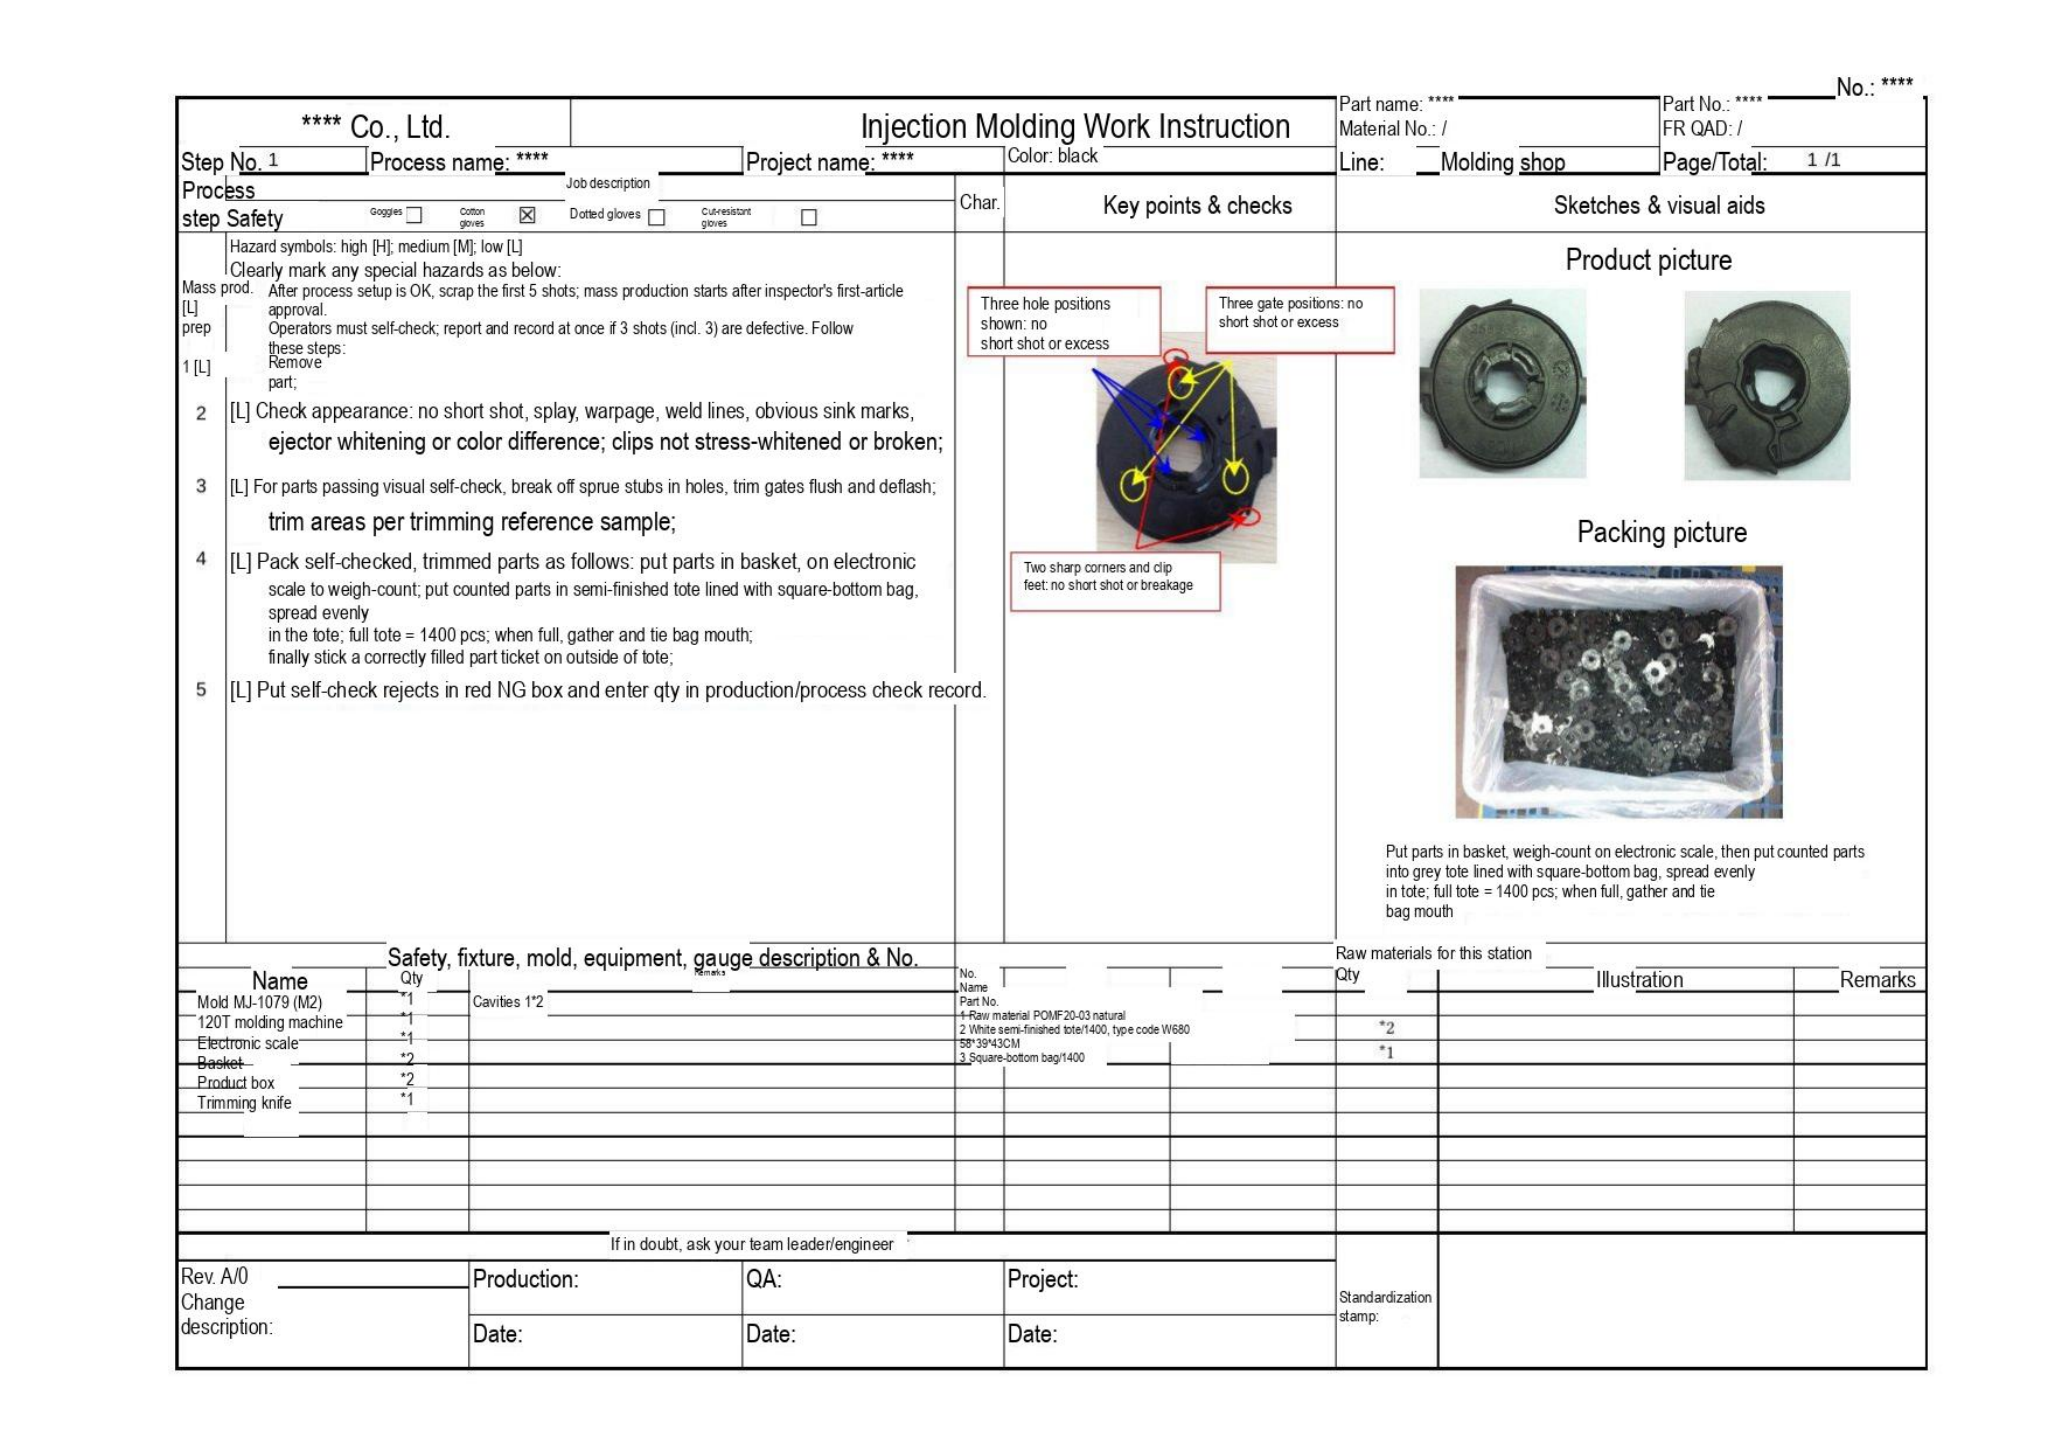No.: ****

**** Co., Ltd.

Injection Molding Work Instruction

Part name: ****
Material No.: /

Part No.: ****
FR QAD: /

Step No. 1 | Process name: **** | Project name: **** | Color: black | Line: Molding shop | Page/Total: 1 /1

Process step | Job description
Safety | Goggles ☐ | Cotton gloves ☒ | Dotted gloves ☐ | Cut-resistant gloves ☐

Char. | Key points & checks | Sketches & visual aids

Hazard symbols: high [H]; medium [M]; low [L]
Clearly mark any special hazards as below:

Mass prod. [L] prep: After process setup is OK, scrap the first 5 shots; mass production starts after inspector's first-article approval.
Operators must self-check; report and record at once if 3 shots (incl. 3) are defective. Follow these steps:

1 [L] Remove part;

2 [L] Check appearance: no short shot, splay, warpage, weld lines, obvious sink marks, ejector whitening or color difference; clips not stress-whitened or broken;

3 [L] For parts passing visual self-check, break off sprue stubs in holes, trim gates flush and deflash; trim areas per trimming reference sample;

4 [L] Pack self-checked, trimmed parts as follows: put parts in basket, on electronic scale to weigh-count; put counted parts in semi-finished tote lined with square-bottom bag, spread evenly
in the tote; full tote = 1400 pcs; when full, gather and tie bag mouth;
finally stick a correctly filled part ticket on outside of tote;

5 [L] Put self-check rejects in red NG box and enter qty in production/process check record.

Three hole positions shown: no short shot or excess

Three gate positions: no short shot or excess

Two sharp corners and clip feet: no short shot or breakage

Product picture

Packing picture

Put parts in basket, weigh-count on electronic scale, then put counted parts into grey tote lined with square-bottom bag, spread evenly
in tote; full tote = 1400 pcs; when full, gather and tie bag mouth

Safety, fixture, mold, equipment, gauge description & No.

| Name | Qty | Remarks |
|---|---|---|
| Mold MJ-1079 (M2) | *1 | Cavities 1*2 |
| 120T molding machine | *1 | |
| Electronic scale | *1 | |
| Basket | *2 | |
| Product box | *2 | |
| Trimming knife | *1 | |

Raw materials for this station

| No. Name Part No. | Qty | Illustration | Remarks |
|---|---|---|---|
| 1 Raw material POMF20-03 natural | | | |
| 2 White semi-finished tote/1400, type code W680 58*39*43CM | *2 | | |
| 3 Square-bottom bag/1400 | *1 | | |

If in doubt, ask your team leader/engineer

| Rev. A/0 Change description: | Production: | QA: | Project: | Standardization stamp: |
|---|---|---|---|---|
| | Date: | Date: | Date: | |